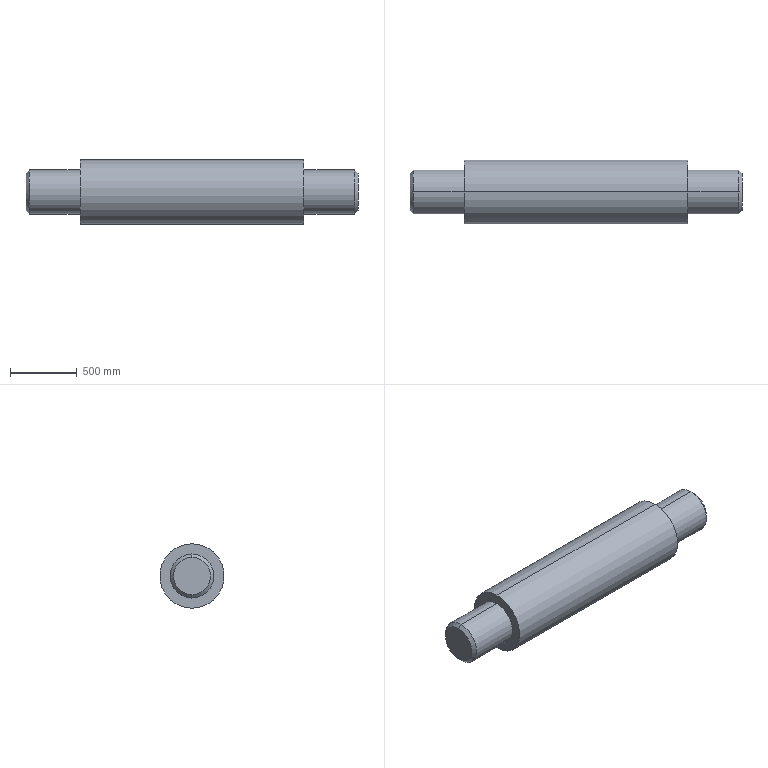Part | SolidWorks | features Chamfer 1, Revolution 1 | 1 solid | 14 faces | box 2489 x 482.6 x 482.6 mm | volume 375617457 mm3 | cylinder 6 | cone 4 | plane 4 | commonest cylinder face diameters 330.2 x4 482.6 x2
STEP:
#1=CARTESIAN_POINT('',(49.,0.,-5.5));
#2=VERTEX_POINT('',#1);
#3=CARTESIAN_POINT('',(49.,0.,5.5));
#4=VERTEX_POINT('',#3);
#5=CARTESIAN_POINT('',(49.,0.,0.));
#6=DIRECTION('',(1.,0.,0.));
#7=DIRECTION('',(0.,0.,1.));
#8=AXIS2_PLACEMENT_3D('',#5,#6,#7);
#9=CIRCLE('',#8,5.5);
#10=EDGE_CURVE('',#2,#4,#9,.T.);
#11=ORIENTED_EDGE('',*,*,#10,.F.);
#12=CARTESIAN_POINT('',(48.,0.,-6.5));
#13=VERTEX_POINT('',#12);
#14=CARTESIAN_POINT('',(48.,0.,-6.5));
#15=DIRECTION('',(-0.7071,0.,-0.7071));
#16=VECTOR('',#15,39.37);
#17=LINE('',#14,#16);
#18=EDGE_CURVE('',#2,#13,#17,.T.);
#19=ORIENTED_EDGE('',*,*,#18,.T.);
#20=CARTESIAN_POINT('',(48.,0.,6.5));
#21=VERTEX_POINT('',#20);
#22=CARTESIAN_POINT('',(48.,0.,0.));
#23=DIRECTION('',(-1.,0.,0.));
#24=DIRECTION('',(0.,0.,1.));
#25=AXIS2_PLACEMENT_3D('',#22,#23,#24);
#26=CIRCLE('',#25,6.5);
#27=EDGE_CURVE('',#21,#13,#26,.T.);
#28=ORIENTED_EDGE('',*,*,#27,.F.);
#29=CARTESIAN_POINT('',(48.,0.,6.5));
#30=DIRECTION('',(-0.7071,0.,0.7071));
#31=VECTOR('',#30,39.37);
#32=LINE('',#29,#31);
#33=EDGE_CURVE('',#4,#21,#32,.T.);
#34=ORIENTED_EDGE('',*,*,#33,.F.);
#35=EDGE_LOOP('',(#11,#19,#28,#34));
#36=FACE_OUTER_BOUND('',#35,.T.);
#37=CARTESIAN_POINT('',(48.,0.,0.));
#38=DIRECTION('',(-1.,0.,0.));
#39=DIRECTION('',(0.,0.,1.));
#40=AXIS2_PLACEMENT_3D('',#37,#38,#39);
#41=CONICAL_SURFACE('',#40,6.5,0.7854);
#42=ADVANCED_FACE('',(#36),#41,.T.);
#43=CARTESIAN_POINT('',(-49.,0.,5.5));
#44=VERTEX_POINT('',#43);
#45=CARTESIAN_POINT('',(-49.,0.,-5.5));
#46=VERTEX_POINT('',#45);
#47=CARTESIAN_POINT('',(-49.,0.,0.));
#48=DIRECTION('',(-1.,0.,0.));
#49=DIRECTION('',(0.,0.,-1.));
#50=AXIS2_PLACEMENT_3D('',#47,#48,#49);
#51=CIRCLE('',#50,5.5);
#52=EDGE_CURVE('',#44,#46,#51,.T.);
#53=ORIENTED_EDGE('',*,*,#52,.F.);
#54=CARTESIAN_POINT('',(-48.,0.,6.5));
#55=VERTEX_POINT('',#54);
#56=CARTESIAN_POINT('',(-49.,0.,5.5));
#57=DIRECTION('',(0.7071,0.,0.7071));
#58=VECTOR('',#57,39.37);
#59=LINE('',#56,#58);
#60=EDGE_CURVE('',#44,#55,#59,.T.);
#61=ORIENTED_EDGE('',*,*,#60,.T.);
#62=CARTESIAN_POINT('',(-48.,0.,-6.5));
#63=VERTEX_POINT('',#62);
#64=CARTESIAN_POINT('',(-48.,0.,0.));
#65=DIRECTION('',(1.,0.,0.));
#66=DIRECTION('',(0.,0.,-1.));
#67=AXIS2_PLACEMENT_3D('',#64,#65,#66);
#68=CIRCLE('',#67,6.5);
#69=EDGE_CURVE('',#63,#55,#68,.T.);
#70=ORIENTED_EDGE('',*,*,#69,.F.);
#71=CARTESIAN_POINT('',(-49.,0.,-5.5));
#72=DIRECTION('',(0.7071,0.,-0.7071));
#73=VECTOR('',#72,39.37);
#74=LINE('',#71,#73);
#75=EDGE_CURVE('',#46,#63,#74,.T.);
#76=ORIENTED_EDGE('',*,*,#75,.F.);
#77=EDGE_LOOP('',(#53,#61,#70,#76));
#78=FACE_OUTER_BOUND('',#77,.T.);
#79=CARTESIAN_POINT('',(-49.,0.,0.));
#80=DIRECTION('',(1.,0.,0.));
#81=DIRECTION('',(0.,0.,-1.));
#82=AXIS2_PLACEMENT_3D('',#79,#80,#81);
#83=CONICAL_SURFACE('',#82,5.5,0.7854);
#84=ADVANCED_FACE('',(#78),#83,.T.);
#85=CARTESIAN_POINT('',(-33.,0.,6.5));
#86=VERTEX_POINT('',#85);
#87=CARTESIAN_POINT('',(-33.,0.,-6.5));
#88=VERTEX_POINT('',#87);
#89=CARTESIAN_POINT('',(-33.,0.,0.));
#90=DIRECTION('',(-1.,0.,0.));
#91=DIRECTION('',(0.,0.,1.));
#92=AXIS2_PLACEMENT_3D('',#89,#90,#91);
#93=CIRCLE('',#92,6.5);
#94=EDGE_CURVE('',#86,#88,#93,.T.);
#95=ORIENTED_EDGE('',*,*,#94,.T.);
#96=CARTESIAN_POINT('',(-49.,0.,-6.5));
#97=DIRECTION('',(-1.,0.,0.));
#98=VECTOR('',#97,39.37);
#99=LINE('',#96,#98);
#100=EDGE_CURVE('',#88,#63,#99,.T.);
#101=ORIENTED_EDGE('',*,*,#100,.T.);
#102=ORIENTED_EDGE('',*,*,#69,.T.);
#103=CARTESIAN_POINT('',(-49.,0.,6.5));
#104=DIRECTION('',(-1.,0.,0.));
#105=VECTOR('',#104,39.37);
#106=LINE('',#103,#105);
#107=EDGE_CURVE('',#86,#55,#106,.T.);
#108=ORIENTED_EDGE('',*,*,#107,.F.);
#109=EDGE_LOOP('',(#95,#101,#102,#108));
#110=FACE_OUTER_BOUND('',#109,.T.);
#111=CARTESIAN_POINT('',(-49.,0.,0.));
#112=DIRECTION('',(-1.,0.,0.));
#113=DIRECTION('',(0.,0.,1.));
#114=AXIS2_PLACEMENT_3D('',#111,#112,#113);
#115=CYLINDRICAL_SURFACE('',#114,6.5);
#116=ADVANCED_FACE('',(#110),#115,.T.);
#117=CARTESIAN_POINT('',(33.,0.,9.5));
#118=VERTEX_POINT('',#117);
#119=CARTESIAN_POINT('',(33.,0.,-9.5));
#120=VERTEX_POINT('',#119);
#121=CARTESIAN_POINT('',(33.,0.,0.));
#122=DIRECTION('',(-1.,0.,0.));
#123=DIRECTION('',(0.,0.,1.));
#124=AXIS2_PLACEMENT_3D('',#121,#122,#123);
#125=CIRCLE('',#124,9.5);
#126=EDGE_CURVE('',#118,#120,#125,.T.);
#127=ORIENTED_EDGE('',*,*,#126,.T.);
#128=CARTESIAN_POINT('',(-33.,0.,-9.5));
#129=VERTEX_POINT('',#128);
#130=CARTESIAN_POINT('',(-49.,0.,-9.5));
#131=DIRECTION('',(-1.,0.,0.));
#132=VECTOR('',#131,39.37);
#133=LINE('',#130,#132);
#134=EDGE_CURVE('',#120,#129,#133,.T.);
#135=ORIENTED_EDGE('',*,*,#134,.T.);
#136=CARTESIAN_POINT('',(-33.,0.,9.5));
#137=VERTEX_POINT('',#136);
#138=CARTESIAN_POINT('',(-33.,0.,0.));
#139=DIRECTION('',(-1.,0.,0.));
#140=DIRECTION('',(0.,0.,1.));
#141=AXIS2_PLACEMENT_3D('',#138,#139,#140);
#142=CIRCLE('',#141,9.5);
#143=EDGE_CURVE('',#137,#129,#142,.T.);
#144=ORIENTED_EDGE('',*,*,#143,.F.);
#145=CARTESIAN_POINT('',(-49.,0.,9.5));
#146=DIRECTION('',(-1.,0.,0.));
#147=VECTOR('',#146,39.37);
#148=LINE('',#145,#147);
#149=EDGE_CURVE('',#118,#137,#148,.T.);
#150=ORIENTED_EDGE('',*,*,#149,.F.);
#151=EDGE_LOOP('',(#127,#135,#144,#150));
#152=FACE_OUTER_BOUND('',#151,.T.);
#153=CARTESIAN_POINT('',(-49.,0.,0.));
#154=DIRECTION('',(-1.,0.,0.));
#155=DIRECTION('',(0.,0.,1.));
#156=AXIS2_PLACEMENT_3D('',#153,#154,#155);
#157=CYLINDRICAL_SURFACE('',#156,9.5);
#158=ADVANCED_FACE('',(#152),#157,.T.);
#159=ORIENTED_EDGE('',*,*,#27,.T.);
#160=CARTESIAN_POINT('',(33.,0.,-6.5));
#161=VERTEX_POINT('',#160);
#162=CARTESIAN_POINT('',(-49.,0.,-6.5));
#163=DIRECTION('',(-1.,0.,0.));
#164=VECTOR('',#163,39.37);
#165=LINE('',#162,#164);
#166=EDGE_CURVE('',#13,#161,#165,.T.);
#167=ORIENTED_EDGE('',*,*,#166,.T.);
#168=CARTESIAN_POINT('',(33.,0.,6.5));
#169=VERTEX_POINT('',#168);
#170=CARTESIAN_POINT('',(33.,0.,0.));
#171=DIRECTION('',(-1.,0.,0.));
#172=DIRECTION('',(0.,0.,1.));
#173=AXIS2_PLACEMENT_3D('',#170,#171,#172);
#174=CIRCLE('',#173,6.5);
#175=EDGE_CURVE('',#169,#161,#174,.T.);
#176=ORIENTED_EDGE('',*,*,#175,.F.);
#177=CARTESIAN_POINT('',(-49.,0.,6.5));
#178=DIRECTION('',(-1.,0.,0.));
#179=VECTOR('',#178,39.37);
#180=LINE('',#177,#179);
#181=EDGE_CURVE('',#21,#169,#180,.T.);
#182=ORIENTED_EDGE('',*,*,#181,.F.);
#183=EDGE_LOOP('',(#159,#167,#176,#182));
#184=FACE_OUTER_BOUND('',#183,.T.);
#185=CARTESIAN_POINT('',(-49.,0.,0.));
#186=DIRECTION('',(-1.,0.,0.));
#187=DIRECTION('',(0.,0.,1.));
#188=AXIS2_PLACEMENT_3D('',#185,#186,#187);
#189=CYLINDRICAL_SURFACE('',#188,6.5);
#190=ADVANCED_FACE('',(#184),#189,.T.);
#191=CARTESIAN_POINT('',(49.,0.,0.));
#192=DIRECTION('',(1.,0.,0.));
#193=DIRECTION('',(0.,0.,1.));
#194=AXIS2_PLACEMENT_3D('',#191,#192,#193);
#195=CIRCLE('',#194,5.5);
#196=EDGE_CURVE('',#4,#2,#195,.T.);
#197=ORIENTED_EDGE('',*,*,#196,.T.);
#198=ORIENTED_EDGE('',*,*,#10,.T.);
#199=EDGE_LOOP('',(#197,#198));
#200=FACE_OUTER_BOUND('',#199,.T.);
#201=CARTESIAN_POINT('',(49.,0.,0.));
#202=DIRECTION('',(-1.,0.,0.));
#203=DIRECTION('',(0.,0.,1.));
#204=AXIS2_PLACEMENT_3D('',#201,#202,#203);
#205=PLANE('',#204);
#206=ADVANCED_FACE('',(#200),#205,.F.);
#207=ORIENTED_EDGE('',*,*,#166,.F.);
#208=CARTESIAN_POINT('',(48.,0.,0.));
#209=DIRECTION('',(-1.,0.,0.));
#210=DIRECTION('',(0.,0.,1.));
#211=AXIS2_PLACEMENT_3D('',#208,#209,#210);
#212=CIRCLE('',#211,6.5);
#213=EDGE_CURVE('',#13,#21,#212,.T.);
#214=ORIENTED_EDGE('',*,*,#213,.T.);
#215=ORIENTED_EDGE('',*,*,#181,.T.);
#216=CARTESIAN_POINT('',(33.,0.,0.));
#217=DIRECTION('',(-1.,0.,0.));
#218=DIRECTION('',(0.,0.,1.));
#219=AXIS2_PLACEMENT_3D('',#216,#217,#218);
#220=CIRCLE('',#219,6.5);
#221=EDGE_CURVE('',#161,#169,#220,.T.);
#222=ORIENTED_EDGE('',*,*,#221,.F.);
#223=EDGE_LOOP('',(#207,#214,#215,#222));
#224=FACE_OUTER_BOUND('',#223,.T.);
#225=CARTESIAN_POINT('',(-49.,0.,0.));
#226=DIRECTION('',(-1.,0.,0.));
#227=DIRECTION('',(0.,0.,1.));
#228=AXIS2_PLACEMENT_3D('',#225,#226,#227);
#229=CYLINDRICAL_SURFACE('',#228,6.5);
#230=ADVANCED_FACE('',(#224),#229,.T.);
#231=ORIENTED_EDGE('',*,*,#126,.F.);
#232=CARTESIAN_POINT('',(33.,0.,0.));
#233=DIRECTION('',(-1.,0.,0.));
#234=DIRECTION('',(0.,0.,1.));
#235=AXIS2_PLACEMENT_3D('',#232,#233,#234);
#236=CIRCLE('',#235,9.5);
#237=EDGE_CURVE('',#120,#118,#236,.T.);
#238=ORIENTED_EDGE('',*,*,#237,.F.);
#239=EDGE_LOOP('',(#231,#238));
#240=FACE_OUTER_BOUND('',#239,.T.);
#241=ORIENTED_EDGE('',*,*,#175,.T.);
#242=ORIENTED_EDGE('',*,*,#221,.T.);
#243=EDGE_LOOP('',(#241,#242));
#244=FACE_BOUND('',#243,.T.);
#245=CARTESIAN_POINT('',(33.,6.5,0.));
#246=DIRECTION('',(-1.,0.,0.));
#247=DIRECTION('',(0.,0.,1.));
#248=AXIS2_PLACEMENT_3D('',#245,#246,#247);
#249=PLANE('',#248);
#250=ADVANCED_FACE('',(#240,#244),#249,.F.);
#251=ORIENTED_EDGE('',*,*,#134,.F.);
#252=ORIENTED_EDGE('',*,*,#237,.T.);
#253=ORIENTED_EDGE('',*,*,#149,.T.);
#254=CARTESIAN_POINT('',(-33.,0.,0.));
#255=DIRECTION('',(-1.,0.,0.));
#256=DIRECTION('',(0.,0.,1.));
#257=AXIS2_PLACEMENT_3D('',#254,#255,#256);
#258=CIRCLE('',#257,9.5);
#259=EDGE_CURVE('',#129,#137,#258,.T.);
#260=ORIENTED_EDGE('',*,*,#259,.F.);
#261=EDGE_LOOP('',(#251,#252,#253,#260));
#262=FACE_OUTER_BOUND('',#261,.T.);
#263=CARTESIAN_POINT('',(-49.,0.,0.));
#264=DIRECTION('',(-1.,0.,0.));
#265=DIRECTION('',(0.,0.,1.));
#266=AXIS2_PLACEMENT_3D('',#263,#264,#265);
#267=CYLINDRICAL_SURFACE('',#266,9.5);
#268=ADVANCED_FACE('',(#262),#267,.T.);
#269=ORIENTED_EDGE('',*,*,#94,.F.);
#270=CARTESIAN_POINT('',(-33.,0.,0.));
#271=DIRECTION('',(-1.,0.,0.));
#272=DIRECTION('',(0.,0.,1.));
#273=AXIS2_PLACEMENT_3D('',#270,#271,#272);
#274=CIRCLE('',#273,6.5);
#275=EDGE_CURVE('',#88,#86,#274,.T.);
#276=ORIENTED_EDGE('',*,*,#275,.F.);
#277=EDGE_LOOP('',(#269,#276));
#278=FACE_BOUND('',#277,.T.);
#279=ORIENTED_EDGE('',*,*,#143,.T.);
#280=ORIENTED_EDGE('',*,*,#259,.T.);
#281=EDGE_LOOP('',(#279,#280));
#282=FACE_OUTER_BOUND('',#281,.T.);
#283=CARTESIAN_POINT('',(-33.,9.5,0.));
#284=DIRECTION('',(1.,0.,0.));
#285=DIRECTION('',(0.,0.,-1.));
#286=AXIS2_PLACEMENT_3D('',#283,#284,#285);
#287=PLANE('',#286);
#288=ADVANCED_FACE('',(#278,#282),#287,.F.);
#289=ORIENTED_EDGE('',*,*,#100,.F.);
#290=ORIENTED_EDGE('',*,*,#275,.T.);
#291=ORIENTED_EDGE('',*,*,#107,.T.);
#292=CARTESIAN_POINT('',(-48.,0.,0.));
#293=DIRECTION('',(1.,0.,0.));
#294=DIRECTION('',(0.,0.,-1.));
#295=AXIS2_PLACEMENT_3D('',#292,#293,#294);
#296=CIRCLE('',#295,6.5);
#297=EDGE_CURVE('',#55,#63,#296,.T.);
#298=ORIENTED_EDGE('',*,*,#297,.T.);
#299=EDGE_LOOP('',(#289,#290,#291,#298));
#300=FACE_OUTER_BOUND('',#299,.T.);
#301=CARTESIAN_POINT('',(-49.,0.,0.));
#302=DIRECTION('',(-1.,0.,0.));
#303=DIRECTION('',(0.,0.,1.));
#304=AXIS2_PLACEMENT_3D('',#301,#302,#303);
#305=CYLINDRICAL_SURFACE('',#304,6.5);
#306=ADVANCED_FACE('',(#300),#305,.T.);
#307=CARTESIAN_POINT('',(-49.,0.,0.));
#308=DIRECTION('',(-1.,0.,0.));
#309=DIRECTION('',(0.,0.,-1.));
#310=AXIS2_PLACEMENT_3D('',#307,#308,#309);
#311=CIRCLE('',#310,5.5);
#312=EDGE_CURVE('',#46,#44,#311,.T.);
#313=ORIENTED_EDGE('',*,*,#312,.T.);
#314=ORIENTED_EDGE('',*,*,#52,.T.);
#315=EDGE_LOOP('',(#313,#314));
#316=FACE_OUTER_BOUND('',#315,.T.);
#317=CARTESIAN_POINT('',(-49.,0.,0.));
#318=DIRECTION('',(1.,0.,0.));
#319=DIRECTION('',(0.,0.,-1.));
#320=AXIS2_PLACEMENT_3D('',#317,#318,#319);
#321=PLANE('',#320);
#322=ADVANCED_FACE('',(#316),#321,.F.);
#323=ORIENTED_EDGE('',*,*,#60,.F.);
#324=ORIENTED_EDGE('',*,*,#312,.F.);
#325=ORIENTED_EDGE('',*,*,#75,.T.);
#326=ORIENTED_EDGE('',*,*,#297,.F.);
#327=EDGE_LOOP('',(#323,#324,#325,#326));
#328=FACE_OUTER_BOUND('',#327,.T.);
#329=CARTESIAN_POINT('',(-49.,0.,0.));
#330=DIRECTION('',(1.,0.,0.));
#331=DIRECTION('',(0.,0.,-1.));
#332=AXIS2_PLACEMENT_3D('',#329,#330,#331);
#333=CONICAL_SURFACE('',#332,5.5,0.7854);
#334=ADVANCED_FACE('',(#328),#333,.T.);
#335=ORIENTED_EDGE('',*,*,#18,.F.);
#336=ORIENTED_EDGE('',*,*,#196,.F.);
#337=ORIENTED_EDGE('',*,*,#33,.T.);
#338=ORIENTED_EDGE('',*,*,#213,.F.);
#339=EDGE_LOOP('',(#335,#336,#337,#338));
#340=FACE_OUTER_BOUND('',#339,.T.);
#341=CARTESIAN_POINT('',(48.,0.,0.));
#342=DIRECTION('',(-1.,0.,0.));
#343=DIRECTION('',(0.,0.,1.));
#344=AXIS2_PLACEMENT_3D('',#341,#342,#343);
#345=CONICAL_SURFACE('',#344,6.5,0.7854);
#346=ADVANCED_FACE('',(#340),#345,.T.);
#347=CLOSED_SHELL('',(#42,#84,#116,#158,#190,#206,#230,#250,#268,#288,#306,#322,#334,#346));
#348=MANIFOLD_SOLID_BREP('',#347);
#349=CARTESIAN_POINT('',(0.,0.,0.));
#350=DIRECTION('',(0.,0.,1.));
#351=DIRECTION('',(1.,0.,0.));
#352=AXIS2_PLACEMENT_3D('',#349,#350,#351);
#353=(LENGTH_UNIT()NAMED_UNIT(*)SI_UNIT($,.METRE.));
#354=LENGTH_MEASURE_WITH_UNIT(LENGTH_MEASURE(0.0254),#353);
#355=DIMENSIONAL_EXPONENTS(1.,0.,0.,0.,0.,0.,0.);
#356=(CONVERSION_BASED_UNIT('INCH',#354)LENGTH_UNIT()NAMED_UNIT(#355));
#357=UNCERTAINTY_MEASURE_WITH_UNIT(LENGTH_MEASURE(0.00001),#356,'','');
#358=(NAMED_UNIT(*)PLANE_ANGLE_UNIT()SI_UNIT($,.RADIAN.));
#359=(NAMED_UNIT(*)SI_UNIT($,.STERADIAN.)SOLID_ANGLE_UNIT());
#360=(GEOMETRIC_REPRESENTATION_CONTEXT(3)GLOBAL_UNCERTAINTY_ASSIGNED_CONTEXT((#357))GLOBAL_UNIT_ASSIGNED_CONTEXT((#356,#358,#359))REPRESENTATION_CONTEXT('',''));
#361=ADVANCED_BREP_SHAPE_REPRESENTATION('',(#348,#352),#360);